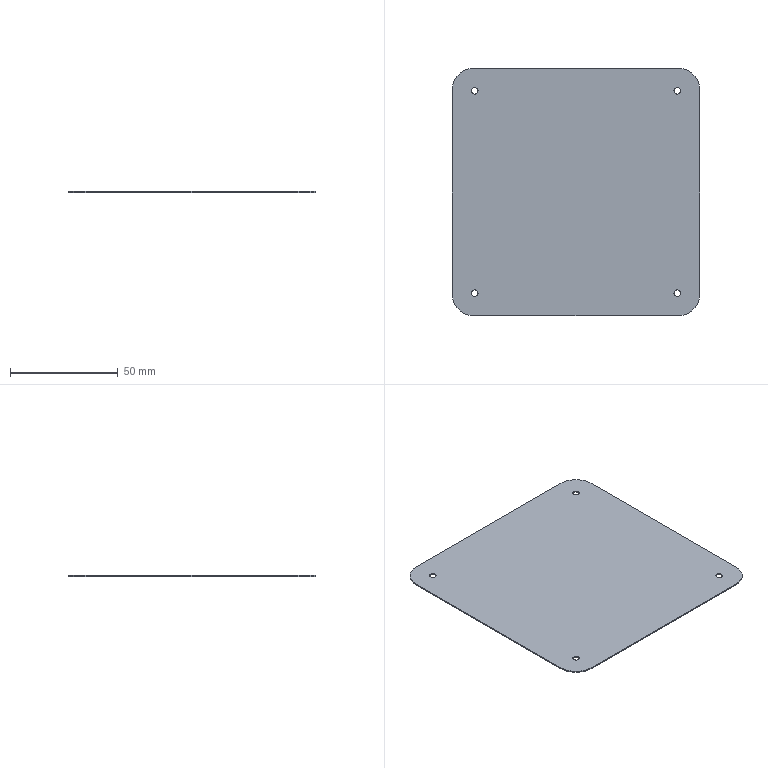Part | SolidWorks | features Extrusion 1 | 1 solid | 18 faces | box 115 x 115 x 0.5 mm | volume 6555 mm3 | cylinder 12 | plane 6 | commonest cylinder face diameters 3 x8 20 x4
STEP:
#1=CARTESIAN_POINT('',(-48.5,-47.,0.5));
#2=VERTEX_POINT('',#1);
#3=CARTESIAN_POINT('',(-45.5,-47.,0.5));
#4=VERTEX_POINT('',#3);
#5=CARTESIAN_POINT('',(-47.,-47.,0.5));
#6=DIRECTION('',(0.,0.,1.));
#7=DIRECTION('',(1.,0.,0.));
#8=AXIS2_PLACEMENT_3D('',#5,#6,#7);
#9=CIRCLE('',#8,1.5);
#10=EDGE_CURVE('',#2,#4,#9,.T.);
#11=ORIENTED_EDGE('',*,*,#10,.T.);
#12=CARTESIAN_POINT('',(-45.5,-47.,0.));
#13=VERTEX_POINT('',#12);
#14=CARTESIAN_POINT('',(-45.5,-47.,0.5));
#15=DIRECTION('',(0.,0.,-1.));
#16=VECTOR('',#15,1000.);
#17=LINE('',#14,#16);
#18=EDGE_CURVE('',#4,#13,#17,.T.);
#19=ORIENTED_EDGE('',*,*,#18,.T.);
#20=CARTESIAN_POINT('',(-48.5,-47.,0.));
#21=VERTEX_POINT('',#20);
#22=CARTESIAN_POINT('',(-47.,-47.,0.));
#23=DIRECTION('',(0.,0.,1.));
#24=DIRECTION('',(1.,0.,0.));
#25=AXIS2_PLACEMENT_3D('',#22,#23,#24);
#26=CIRCLE('',#25,1.5);
#27=EDGE_CURVE('',#21,#13,#26,.T.);
#28=ORIENTED_EDGE('',*,*,#27,.F.);
#29=CARTESIAN_POINT('',(-48.5,-47.,0.5));
#30=DIRECTION('',(0.,0.,-1.));
#31=VECTOR('',#30,1000.);
#32=LINE('',#29,#31);
#33=EDGE_CURVE('',#2,#21,#32,.T.);
#34=ORIENTED_EDGE('',*,*,#33,.F.);
#35=EDGE_LOOP('',(#11,#19,#28,#34));
#36=FACE_OUTER_BOUND('',#35,.T.);
#37=CARTESIAN_POINT('',(-47.,-47.,0.5));
#38=DIRECTION('',(0.,0.,-1.));
#39=DIRECTION('',(-1.,0.,0.));
#40=AXIS2_PLACEMENT_3D('',#37,#38,#39);
#41=CYLINDRICAL_SURFACE('',#40,1.5);
#42=ADVANCED_FACE('',(#36),#41,.F.);
#43=CARTESIAN_POINT('',(45.5,-47.,0.5));
#44=VERTEX_POINT('',#43);
#45=CARTESIAN_POINT('',(48.5,-47.,0.5));
#46=VERTEX_POINT('',#45);
#47=CARTESIAN_POINT('',(47.,-47.,0.5));
#48=DIRECTION('',(0.,0.,1.));
#49=DIRECTION('',(1.,0.,0.));
#50=AXIS2_PLACEMENT_3D('',#47,#48,#49);
#51=CIRCLE('',#50,1.5);
#52=EDGE_CURVE('',#44,#46,#51,.T.);
#53=ORIENTED_EDGE('',*,*,#52,.T.);
#54=CARTESIAN_POINT('',(48.5,-47.,0.));
#55=VERTEX_POINT('',#54);
#56=CARTESIAN_POINT('',(48.5,-47.,0.5));
#57=DIRECTION('',(0.,0.,-1.));
#58=VECTOR('',#57,1000.);
#59=LINE('',#56,#58);
#60=EDGE_CURVE('',#46,#55,#59,.T.);
#61=ORIENTED_EDGE('',*,*,#60,.T.);
#62=CARTESIAN_POINT('',(45.5,-47.,0.));
#63=VERTEX_POINT('',#62);
#64=CARTESIAN_POINT('',(47.,-47.,0.));
#65=DIRECTION('',(0.,0.,1.));
#66=DIRECTION('',(1.,0.,0.));
#67=AXIS2_PLACEMENT_3D('',#64,#65,#66);
#68=CIRCLE('',#67,1.5);
#69=EDGE_CURVE('',#63,#55,#68,.T.);
#70=ORIENTED_EDGE('',*,*,#69,.F.);
#71=CARTESIAN_POINT('',(45.5,-47.,0.5));
#72=DIRECTION('',(0.,0.,-1.));
#73=VECTOR('',#72,1000.);
#74=LINE('',#71,#73);
#75=EDGE_CURVE('',#44,#63,#74,.T.);
#76=ORIENTED_EDGE('',*,*,#75,.F.);
#77=EDGE_LOOP('',(#53,#61,#70,#76));
#78=FACE_OUTER_BOUND('',#77,.T.);
#79=CARTESIAN_POINT('',(47.,-47.,0.5));
#80=DIRECTION('',(0.,0.,-1.));
#81=DIRECTION('',(-1.,0.,0.));
#82=AXIS2_PLACEMENT_3D('',#79,#80,#81);
#83=CYLINDRICAL_SURFACE('',#82,1.5);
#84=ADVANCED_FACE('',(#78),#83,.F.);
#85=CARTESIAN_POINT('',(45.5,47.,0.5));
#86=VERTEX_POINT('',#85);
#87=CARTESIAN_POINT('',(48.5,47.,0.5));
#88=VERTEX_POINT('',#87);
#89=CARTESIAN_POINT('',(47.,47.,0.5));
#90=DIRECTION('',(0.,0.,1.));
#91=DIRECTION('',(1.,0.,0.));
#92=AXIS2_PLACEMENT_3D('',#89,#90,#91);
#93=CIRCLE('',#92,1.5);
#94=EDGE_CURVE('',#86,#88,#93,.T.);
#95=ORIENTED_EDGE('',*,*,#94,.T.);
#96=CARTESIAN_POINT('',(48.5,47.,0.));
#97=VERTEX_POINT('',#96);
#98=CARTESIAN_POINT('',(48.5,47.,0.5));
#99=DIRECTION('',(0.,0.,-1.));
#100=VECTOR('',#99,1000.);
#101=LINE('',#98,#100);
#102=EDGE_CURVE('',#88,#97,#101,.T.);
#103=ORIENTED_EDGE('',*,*,#102,.T.);
#104=CARTESIAN_POINT('',(45.5,47.,0.));
#105=VERTEX_POINT('',#104);
#106=CARTESIAN_POINT('',(47.,47.,0.));
#107=DIRECTION('',(0.,0.,1.));
#108=DIRECTION('',(1.,0.,0.));
#109=AXIS2_PLACEMENT_3D('',#106,#107,#108);
#110=CIRCLE('',#109,1.5);
#111=EDGE_CURVE('',#105,#97,#110,.T.);
#112=ORIENTED_EDGE('',*,*,#111,.F.);
#113=CARTESIAN_POINT('',(45.5,47.,0.5));
#114=DIRECTION('',(0.,0.,-1.));
#115=VECTOR('',#114,1000.);
#116=LINE('',#113,#115);
#117=EDGE_CURVE('',#86,#105,#116,.T.);
#118=ORIENTED_EDGE('',*,*,#117,.F.);
#119=EDGE_LOOP('',(#95,#103,#112,#118));
#120=FACE_OUTER_BOUND('',#119,.T.);
#121=CARTESIAN_POINT('',(47.,47.,0.5));
#122=DIRECTION('',(0.,0.,-1.));
#123=DIRECTION('',(-1.,0.,0.));
#124=AXIS2_PLACEMENT_3D('',#121,#122,#123);
#125=CYLINDRICAL_SURFACE('',#124,1.5);
#126=ADVANCED_FACE('',(#120),#125,.F.);
#127=CARTESIAN_POINT('',(-48.5,47.,0.5));
#128=VERTEX_POINT('',#127);
#129=CARTESIAN_POINT('',(-45.5,47.,0.5));
#130=VERTEX_POINT('',#129);
#131=CARTESIAN_POINT('',(-47.,47.,0.5));
#132=DIRECTION('',(0.,0.,1.));
#133=DIRECTION('',(1.,0.,0.));
#134=AXIS2_PLACEMENT_3D('',#131,#132,#133);
#135=CIRCLE('',#134,1.5);
#136=EDGE_CURVE('',#128,#130,#135,.T.);
#137=ORIENTED_EDGE('',*,*,#136,.T.);
#138=CARTESIAN_POINT('',(-45.5,47.,0.));
#139=VERTEX_POINT('',#138);
#140=CARTESIAN_POINT('',(-45.5,47.,0.5));
#141=DIRECTION('',(0.,0.,-1.));
#142=VECTOR('',#141,1000.);
#143=LINE('',#140,#142);
#144=EDGE_CURVE('',#130,#139,#143,.T.);
#145=ORIENTED_EDGE('',*,*,#144,.T.);
#146=CARTESIAN_POINT('',(-48.5,47.,0.));
#147=VERTEX_POINT('',#146);
#148=CARTESIAN_POINT('',(-47.,47.,0.));
#149=DIRECTION('',(0.,0.,1.));
#150=DIRECTION('',(1.,0.,0.));
#151=AXIS2_PLACEMENT_3D('',#148,#149,#150);
#152=CIRCLE('',#151,1.5);
#153=EDGE_CURVE('',#147,#139,#152,.T.);
#154=ORIENTED_EDGE('',*,*,#153,.F.);
#155=CARTESIAN_POINT('',(-48.5,47.,0.5));
#156=DIRECTION('',(0.,0.,-1.));
#157=VECTOR('',#156,1000.);
#158=LINE('',#155,#157);
#159=EDGE_CURVE('',#128,#147,#158,.T.);
#160=ORIENTED_EDGE('',*,*,#159,.F.);
#161=EDGE_LOOP('',(#137,#145,#154,#160));
#162=FACE_OUTER_BOUND('',#161,.T.);
#163=CARTESIAN_POINT('',(-47.,47.,0.5));
#164=DIRECTION('',(0.,0.,-1.));
#165=DIRECTION('',(-1.,0.,0.));
#166=AXIS2_PLACEMENT_3D('',#163,#164,#165);
#167=CYLINDRICAL_SURFACE('',#166,1.5);
#168=ADVANCED_FACE('',(#162),#167,.F.);
#169=ORIENTED_EDGE('',*,*,#52,.F.);
#170=CARTESIAN_POINT('',(47.,-47.,0.5));
#171=DIRECTION('',(0.,0.,1.));
#172=DIRECTION('',(1.,0.,0.));
#173=AXIS2_PLACEMENT_3D('',#170,#171,#172);
#174=CIRCLE('',#173,1.5);
#175=EDGE_CURVE('',#46,#44,#174,.T.);
#176=ORIENTED_EDGE('',*,*,#175,.F.);
#177=EDGE_LOOP('',(#169,#176));
#178=FACE_BOUND('',#177,.T.);
#179=ORIENTED_EDGE('',*,*,#136,.F.);
#180=CARTESIAN_POINT('',(-47.,47.,0.5));
#181=DIRECTION('',(0.,0.,1.));
#182=DIRECTION('',(1.,0.,0.));
#183=AXIS2_PLACEMENT_3D('',#180,#181,#182);
#184=CIRCLE('',#183,1.5);
#185=EDGE_CURVE('',#130,#128,#184,.T.);
#186=ORIENTED_EDGE('',*,*,#185,.F.);
#187=EDGE_LOOP('',(#179,#186));
#188=FACE_BOUND('',#187,.T.);
#189=CARTESIAN_POINT('',(-47.5,57.5,0.5));
#190=VERTEX_POINT('',#189);
#191=CARTESIAN_POINT('',(-57.5,47.5,0.5));
#192=VERTEX_POINT('',#191);
#193=CARTESIAN_POINT('',(-47.5,47.5,0.5));
#194=DIRECTION('',(0.,0.,1.));
#195=DIRECTION('',(1.,0.,0.));
#196=AXIS2_PLACEMENT_3D('',#193,#194,#195);
#197=CIRCLE('',#196,10.);
#198=EDGE_CURVE('',#190,#192,#197,.T.);
#199=ORIENTED_EDGE('',*,*,#198,.T.);
#200=CARTESIAN_POINT('',(-57.5,-47.5,0.5));
#201=VERTEX_POINT('',#200);
#202=CARTESIAN_POINT('',(-57.5,47.5,0.5));
#203=DIRECTION('',(0.,-1.,0.));
#204=VECTOR('',#203,1000.);
#205=LINE('',#202,#204);
#206=EDGE_CURVE('',#192,#201,#205,.T.);
#207=ORIENTED_EDGE('',*,*,#206,.T.);
#208=CARTESIAN_POINT('',(-47.5,-57.5,0.5));
#209=VERTEX_POINT('',#208);
#210=CARTESIAN_POINT('',(-47.5,-47.5,0.5));
#211=DIRECTION('',(0.,0.,1.));
#212=DIRECTION('',(-1.,0.,0.));
#213=AXIS2_PLACEMENT_3D('',#210,#211,#212);
#214=CIRCLE('',#213,10.);
#215=EDGE_CURVE('',#201,#209,#214,.T.);
#216=ORIENTED_EDGE('',*,*,#215,.T.);
#217=CARTESIAN_POINT('',(47.5,-57.5,0.5));
#218=VERTEX_POINT('',#217);
#219=CARTESIAN_POINT('',(47.5,-57.5,0.5));
#220=DIRECTION('',(1.,0.,0.));
#221=VECTOR('',#220,1000.);
#222=LINE('',#219,#221);
#223=EDGE_CURVE('',#209,#218,#222,.T.);
#224=ORIENTED_EDGE('',*,*,#223,.T.);
#225=CARTESIAN_POINT('',(57.5,-47.5,0.5));
#226=VERTEX_POINT('',#225);
#227=CARTESIAN_POINT('',(47.5,-47.5,0.5));
#228=DIRECTION('',(0.,0.,1.));
#229=DIRECTION('',(-1.,0.,0.));
#230=AXIS2_PLACEMENT_3D('',#227,#228,#229);
#231=CIRCLE('',#230,10.);
#232=EDGE_CURVE('',#218,#226,#231,.T.);
#233=ORIENTED_EDGE('',*,*,#232,.T.);
#234=CARTESIAN_POINT('',(57.5,47.5,0.5));
#235=VERTEX_POINT('',#234);
#236=CARTESIAN_POINT('',(57.5,47.5,0.5));
#237=DIRECTION('',(0.,1.,0.));
#238=VECTOR('',#237,1000.);
#239=LINE('',#236,#238);
#240=EDGE_CURVE('',#226,#235,#239,.T.);
#241=ORIENTED_EDGE('',*,*,#240,.T.);
#242=CARTESIAN_POINT('',(47.5,57.5,0.5));
#243=VERTEX_POINT('',#242);
#244=CARTESIAN_POINT('',(47.5,47.5,0.5));
#245=DIRECTION('',(0.,0.,1.));
#246=DIRECTION('',(-1.,0.,0.));
#247=AXIS2_PLACEMENT_3D('',#244,#245,#246);
#248=CIRCLE('',#247,10.);
#249=EDGE_CURVE('',#235,#243,#248,.T.);
#250=ORIENTED_EDGE('',*,*,#249,.T.);
#251=CARTESIAN_POINT('',(47.5,57.5,0.5));
#252=DIRECTION('',(-1.,0.,0.));
#253=VECTOR('',#252,1000.);
#254=LINE('',#251,#253);
#255=EDGE_CURVE('',#243,#190,#254,.T.);
#256=ORIENTED_EDGE('',*,*,#255,.T.);
#257=EDGE_LOOP('',(#199,#207,#216,#224,#233,#241,#250,#256));
#258=FACE_OUTER_BOUND('',#257,.T.);
#259=ORIENTED_EDGE('',*,*,#94,.F.);
#260=CARTESIAN_POINT('',(47.,47.,0.5));
#261=DIRECTION('',(0.,0.,1.));
#262=DIRECTION('',(1.,0.,0.));
#263=AXIS2_PLACEMENT_3D('',#260,#261,#262);
#264=CIRCLE('',#263,1.5);
#265=EDGE_CURVE('',#88,#86,#264,.T.);
#266=ORIENTED_EDGE('',*,*,#265,.F.);
#267=EDGE_LOOP('',(#259,#266));
#268=FACE_BOUND('',#267,.T.);
#269=ORIENTED_EDGE('',*,*,#10,.F.);
#270=CARTESIAN_POINT('',(-47.,-47.,0.5));
#271=DIRECTION('',(0.,0.,1.));
#272=DIRECTION('',(1.,0.,0.));
#273=AXIS2_PLACEMENT_3D('',#270,#271,#272);
#274=CIRCLE('',#273,1.5);
#275=EDGE_CURVE('',#4,#2,#274,.T.);
#276=ORIENTED_EDGE('',*,*,#275,.F.);
#277=EDGE_LOOP('',(#269,#276));
#278=FACE_BOUND('',#277,.T.);
#279=CARTESIAN_POINT('',(-47.5,47.5,0.5));
#280=DIRECTION('',(0.,0.,1.));
#281=DIRECTION('',(1.,0.,0.));
#282=AXIS2_PLACEMENT_3D('',#279,#280,#281);
#283=PLANE('',#282);
#284=ADVANCED_FACE('',(#178,#188,#258,#268,#278),#283,.T.);
#285=CARTESIAN_POINT('',(-47.5,57.5,0.));
#286=VERTEX_POINT('',#285);
#287=CARTESIAN_POINT('',(-57.5,47.5,0.));
#288=VERTEX_POINT('',#287);
#289=CARTESIAN_POINT('',(-47.5,47.5,0.));
#290=DIRECTION('',(0.,0.,1.));
#291=DIRECTION('',(1.,0.,0.));
#292=AXIS2_PLACEMENT_3D('',#289,#290,#291);
#293=CIRCLE('',#292,10.);
#294=EDGE_CURVE('',#286,#288,#293,.T.);
#295=ORIENTED_EDGE('',*,*,#294,.F.);
#296=CARTESIAN_POINT('',(47.5,57.5,0.));
#297=VERTEX_POINT('',#296);
#298=CARTESIAN_POINT('',(47.5,57.5,0.));
#299=DIRECTION('',(-1.,0.,0.));
#300=VECTOR('',#299,1000.);
#301=LINE('',#298,#300);
#302=EDGE_CURVE('',#297,#286,#301,.T.);
#303=ORIENTED_EDGE('',*,*,#302,.F.);
#304=CARTESIAN_POINT('',(57.5,47.5,0.));
#305=VERTEX_POINT('',#304);
#306=CARTESIAN_POINT('',(47.5,47.5,0.));
#307=DIRECTION('',(0.,0.,1.));
#308=DIRECTION('',(-1.,0.,0.));
#309=AXIS2_PLACEMENT_3D('',#306,#307,#308);
#310=CIRCLE('',#309,10.);
#311=EDGE_CURVE('',#305,#297,#310,.T.);
#312=ORIENTED_EDGE('',*,*,#311,.F.);
#313=CARTESIAN_POINT('',(57.5,-47.5,0.));
#314=VERTEX_POINT('',#313);
#315=CARTESIAN_POINT('',(57.5,47.5,0.));
#316=DIRECTION('',(0.,1.,0.));
#317=VECTOR('',#316,1000.);
#318=LINE('',#315,#317);
#319=EDGE_CURVE('',#314,#305,#318,.T.);
#320=ORIENTED_EDGE('',*,*,#319,.F.);
#321=CARTESIAN_POINT('',(47.5,-57.5,0.));
#322=VERTEX_POINT('',#321);
#323=CARTESIAN_POINT('',(47.5,-47.5,0.));
#324=DIRECTION('',(0.,0.,1.));
#325=DIRECTION('',(-1.,0.,0.));
#326=AXIS2_PLACEMENT_3D('',#323,#324,#325);
#327=CIRCLE('',#326,10.);
#328=EDGE_CURVE('',#322,#314,#327,.T.);
#329=ORIENTED_EDGE('',*,*,#328,.F.);
#330=CARTESIAN_POINT('',(-47.5,-57.5,0.));
#331=VERTEX_POINT('',#330);
#332=CARTESIAN_POINT('',(47.5,-57.5,0.));
#333=DIRECTION('',(1.,0.,0.));
#334=VECTOR('',#333,1000.);
#335=LINE('',#332,#334);
#336=EDGE_CURVE('',#331,#322,#335,.T.);
#337=ORIENTED_EDGE('',*,*,#336,.F.);
#338=CARTESIAN_POINT('',(-57.5,-47.5,0.));
#339=VERTEX_POINT('',#338);
#340=CARTESIAN_POINT('',(-47.5,-47.5,0.));
#341=DIRECTION('',(0.,0.,1.));
#342=DIRECTION('',(-1.,0.,0.));
#343=AXIS2_PLACEMENT_3D('',#340,#341,#342);
#344=CIRCLE('',#343,10.);
#345=EDGE_CURVE('',#339,#331,#344,.T.);
#346=ORIENTED_EDGE('',*,*,#345,.F.);
#347=CARTESIAN_POINT('',(-57.5,47.5,0.));
#348=DIRECTION('',(0.,-1.,0.));
#349=VECTOR('',#348,1000.);
#350=LINE('',#347,#349);
#351=EDGE_CURVE('',#288,#339,#350,.T.);
#352=ORIENTED_EDGE('',*,*,#351,.F.);
#353=EDGE_LOOP('',(#295,#303,#312,#320,#329,#337,#346,#352));
#354=FACE_OUTER_BOUND('',#353,.T.);
#355=ORIENTED_EDGE('',*,*,#153,.T.);
#356=CARTESIAN_POINT('',(-47.,47.,0.));
#357=DIRECTION('',(0.,0.,1.));
#358=DIRECTION('',(1.,0.,0.));
#359=AXIS2_PLACEMENT_3D('',#356,#357,#358);
#360=CIRCLE('',#359,1.5);
#361=EDGE_CURVE('',#139,#147,#360,.T.);
#362=ORIENTED_EDGE('',*,*,#361,.T.);
#363=EDGE_LOOP('',(#355,#362));
#364=FACE_BOUND('',#363,.T.);
#365=ORIENTED_EDGE('',*,*,#111,.T.);
#366=CARTESIAN_POINT('',(47.,47.,0.));
#367=DIRECTION('',(0.,0.,1.));
#368=DIRECTION('',(1.,0.,0.));
#369=AXIS2_PLACEMENT_3D('',#366,#367,#368);
#370=CIRCLE('',#369,1.5);
#371=EDGE_CURVE('',#97,#105,#370,.T.);
#372=ORIENTED_EDGE('',*,*,#371,.T.);
#373=EDGE_LOOP('',(#365,#372));
#374=FACE_BOUND('',#373,.T.);
#375=ORIENTED_EDGE('',*,*,#69,.T.);
#376=CARTESIAN_POINT('',(47.,-47.,0.));
#377=DIRECTION('',(0.,0.,1.));
#378=DIRECTION('',(1.,0.,0.));
#379=AXIS2_PLACEMENT_3D('',#376,#377,#378);
#380=CIRCLE('',#379,1.5);
#381=EDGE_CURVE('',#55,#63,#380,.T.);
#382=ORIENTED_EDGE('',*,*,#381,.T.);
#383=EDGE_LOOP('',(#375,#382));
#384=FACE_BOUND('',#383,.T.);
#385=ORIENTED_EDGE('',*,*,#27,.T.);
#386=CARTESIAN_POINT('',(-47.,-47.,0.));
#387=DIRECTION('',(0.,0.,1.));
#388=DIRECTION('',(1.,0.,0.));
#389=AXIS2_PLACEMENT_3D('',#386,#387,#388);
#390=CIRCLE('',#389,1.5);
#391=EDGE_CURVE('',#13,#21,#390,.T.);
#392=ORIENTED_EDGE('',*,*,#391,.T.);
#393=EDGE_LOOP('',(#385,#392));
#394=FACE_BOUND('',#393,.T.);
#395=CARTESIAN_POINT('',(-47.5,47.5,0.));
#396=DIRECTION('',(0.,0.,1.));
#397=DIRECTION('',(1.,0.,0.));
#398=AXIS2_PLACEMENT_3D('',#395,#396,#397);
#399=PLANE('',#398);
#400=ADVANCED_FACE('',(#354,#364,#374,#384,#394),#399,.F.);
#401=ORIENTED_EDGE('',*,*,#294,.T.);
#402=CARTESIAN_POINT('',(-57.5,47.5,0.5));
#403=DIRECTION('',(0.,0.,-1.));
#404=VECTOR('',#403,1000.);
#405=LINE('',#402,#404);
#406=EDGE_CURVE('',#192,#288,#405,.T.);
#407=ORIENTED_EDGE('',*,*,#406,.F.);
#408=ORIENTED_EDGE('',*,*,#198,.F.);
#409=CARTESIAN_POINT('',(-47.5,57.5,0.5));
#410=DIRECTION('',(0.,0.,-1.));
#411=VECTOR('',#410,1000.);
#412=LINE('',#409,#411);
#413=EDGE_CURVE('',#190,#286,#412,.T.);
#414=ORIENTED_EDGE('',*,*,#413,.T.);
#415=EDGE_LOOP('',(#401,#407,#408,#414));
#416=FACE_OUTER_BOUND('',#415,.T.);
#417=CARTESIAN_POINT('',(-47.5,47.5,0.5));
#418=DIRECTION('',(0.,0.,-1.));
#419=DIRECTION('',(-1.,0.,0.));
#420=AXIS2_PLACEMENT_3D('',#417,#418,#419);
#421=CYLINDRICAL_SURFACE('',#420,10.);
#422=ADVANCED_FACE('',(#416),#421,.T.);
#423=ORIENTED_EDGE('',*,*,#351,.T.);
#424=CARTESIAN_POINT('',(-57.5,-47.5,0.5));
#425=DIRECTION('',(0.,0.,-1.));
#426=VECTOR('',#425,1000.);
#427=LINE('',#424,#426);
#428=EDGE_CURVE('',#201,#339,#427,.T.);
#429=ORIENTED_EDGE('',*,*,#428,.F.);
#430=ORIENTED_EDGE('',*,*,#206,.F.);
#431=ORIENTED_EDGE('',*,*,#406,.T.);
#432=EDGE_LOOP('',(#423,#429,#430,#431));
#433=FACE_OUTER_BOUND('',#432,.T.);
#434=CARTESIAN_POINT('',(-57.5,47.5,0.5));
#435=DIRECTION('',(1.,0.,0.));
#436=DIRECTION('',(0.,1.,0.));
#437=AXIS2_PLACEMENT_3D('',#434,#435,#436);
#438=PLANE('',#437);
#439=ADVANCED_FACE('',(#433),#438,.F.);
#440=ORIENTED_EDGE('',*,*,#345,.T.);
#441=CARTESIAN_POINT('',(-47.5,-57.5,0.5));
#442=DIRECTION('',(0.,0.,-1.));
#443=VECTOR('',#442,1000.);
#444=LINE('',#441,#443);
#445=EDGE_CURVE('',#209,#331,#444,.T.);
#446=ORIENTED_EDGE('',*,*,#445,.F.);
#447=ORIENTED_EDGE('',*,*,#215,.F.);
#448=ORIENTED_EDGE('',*,*,#428,.T.);
#449=EDGE_LOOP('',(#440,#446,#447,#448));
#450=FACE_OUTER_BOUND('',#449,.T.);
#451=CARTESIAN_POINT('',(-47.5,-47.5,0.5));
#452=DIRECTION('',(0.,0.,-1.));
#453=DIRECTION('',(-1.,0.,0.));
#454=AXIS2_PLACEMENT_3D('',#451,#452,#453);
#455=CYLINDRICAL_SURFACE('',#454,10.);
#456=ADVANCED_FACE('',(#450),#455,.T.);
#457=ORIENTED_EDGE('',*,*,#336,.T.);
#458=CARTESIAN_POINT('',(47.5,-57.5,0.5));
#459=DIRECTION('',(0.,0.,-1.));
#460=VECTOR('',#459,1000.);
#461=LINE('',#458,#460);
#462=EDGE_CURVE('',#218,#322,#461,.T.);
#463=ORIENTED_EDGE('',*,*,#462,.F.);
#464=ORIENTED_EDGE('',*,*,#223,.F.);
#465=ORIENTED_EDGE('',*,*,#445,.T.);
#466=EDGE_LOOP('',(#457,#463,#464,#465));
#467=FACE_OUTER_BOUND('',#466,.T.);
#468=CARTESIAN_POINT('',(47.5,-57.5,0.5));
#469=DIRECTION('',(0.,1.,0.));
#470=DIRECTION('',(-1.,0.,0.));
#471=AXIS2_PLACEMENT_3D('',#468,#469,#470);
#472=PLANE('',#471);
#473=ADVANCED_FACE('',(#467),#472,.F.);
#474=ORIENTED_EDGE('',*,*,#328,.T.);
#475=CARTESIAN_POINT('',(57.5,-47.5,0.5));
#476=DIRECTION('',(0.,0.,-1.));
#477=VECTOR('',#476,1000.);
#478=LINE('',#475,#477);
#479=EDGE_CURVE('',#226,#314,#478,.T.);
#480=ORIENTED_EDGE('',*,*,#479,.F.);
#481=ORIENTED_EDGE('',*,*,#232,.F.);
#482=ORIENTED_EDGE('',*,*,#462,.T.);
#483=EDGE_LOOP('',(#474,#480,#481,#482));
#484=FACE_OUTER_BOUND('',#483,.T.);
#485=CARTESIAN_POINT('',(47.5,-47.5,0.5));
#486=DIRECTION('',(0.,0.,-1.));
#487=DIRECTION('',(-1.,0.,0.));
#488=AXIS2_PLACEMENT_3D('',#485,#486,#487);
#489=CYLINDRICAL_SURFACE('',#488,10.);
#490=ADVANCED_FACE('',(#484),#489,.T.);
#491=ORIENTED_EDGE('',*,*,#319,.T.);
#492=CARTESIAN_POINT('',(57.5,47.5,0.5));
#493=DIRECTION('',(0.,0.,-1.));
#494=VECTOR('',#493,1000.);
#495=LINE('',#492,#494);
#496=EDGE_CURVE('',#235,#305,#495,.T.);
#497=ORIENTED_EDGE('',*,*,#496,.F.);
#498=ORIENTED_EDGE('',*,*,#240,.F.);
#499=ORIENTED_EDGE('',*,*,#479,.T.);
#500=EDGE_LOOP('',(#491,#497,#498,#499));
#501=FACE_OUTER_BOUND('',#500,.T.);
#502=CARTESIAN_POINT('',(57.5,47.5,0.5));
#503=DIRECTION('',(-1.,0.,0.));
#504=DIRECTION('',(0.,-1.,0.));
#505=AXIS2_PLACEMENT_3D('',#502,#503,#504);
#506=PLANE('',#505);
#507=ADVANCED_FACE('',(#501),#506,.F.);
#508=ORIENTED_EDGE('',*,*,#311,.T.);
#509=CARTESIAN_POINT('',(47.5,57.5,0.5));
#510=DIRECTION('',(0.,0.,-1.));
#511=VECTOR('',#510,1000.);
#512=LINE('',#509,#511);
#513=EDGE_CURVE('',#243,#297,#512,.T.);
#514=ORIENTED_EDGE('',*,*,#513,.F.);
#515=ORIENTED_EDGE('',*,*,#249,.F.);
#516=ORIENTED_EDGE('',*,*,#496,.T.);
#517=EDGE_LOOP('',(#508,#514,#515,#516));
#518=FACE_OUTER_BOUND('',#517,.T.);
#519=CARTESIAN_POINT('',(47.5,47.5,0.5));
#520=DIRECTION('',(0.,0.,-1.));
#521=DIRECTION('',(-1.,0.,0.));
#522=AXIS2_PLACEMENT_3D('',#519,#520,#521);
#523=CYLINDRICAL_SURFACE('',#522,10.);
#524=ADVANCED_FACE('',(#518),#523,.T.);
#525=ORIENTED_EDGE('',*,*,#302,.T.);
#526=ORIENTED_EDGE('',*,*,#413,.F.);
#527=ORIENTED_EDGE('',*,*,#255,.F.);
#528=ORIENTED_EDGE('',*,*,#513,.T.);
#529=EDGE_LOOP('',(#525,#526,#527,#528));
#530=FACE_OUTER_BOUND('',#529,.T.);
#531=CARTESIAN_POINT('',(47.5,57.5,0.5));
#532=DIRECTION('',(0.,-1.,0.));
#533=DIRECTION('',(1.,0.,0.));
#534=AXIS2_PLACEMENT_3D('',#531,#532,#533);
#535=PLANE('',#534);
#536=ADVANCED_FACE('',(#530),#535,.F.);
#537=ORIENTED_EDGE('',*,*,#144,.F.);
#538=ORIENTED_EDGE('',*,*,#185,.T.);
#539=ORIENTED_EDGE('',*,*,#159,.T.);
#540=ORIENTED_EDGE('',*,*,#361,.F.);
#541=EDGE_LOOP('',(#537,#538,#539,#540));
#542=FACE_OUTER_BOUND('',#541,.T.);
#543=CARTESIAN_POINT('',(-47.,47.,0.5));
#544=DIRECTION('',(0.,0.,-1.));
#545=DIRECTION('',(-1.,0.,0.));
#546=AXIS2_PLACEMENT_3D('',#543,#544,#545);
#547=CYLINDRICAL_SURFACE('',#546,1.5);
#548=ADVANCED_FACE('',(#542),#547,.F.);
#549=ORIENTED_EDGE('',*,*,#102,.F.);
#550=ORIENTED_EDGE('',*,*,#265,.T.);
#551=ORIENTED_EDGE('',*,*,#117,.T.);
#552=ORIENTED_EDGE('',*,*,#371,.F.);
#553=EDGE_LOOP('',(#549,#550,#551,#552));
#554=FACE_OUTER_BOUND('',#553,.T.);
#555=CARTESIAN_POINT('',(47.,47.,0.5));
#556=DIRECTION('',(0.,0.,-1.));
#557=DIRECTION('',(-1.,0.,0.));
#558=AXIS2_PLACEMENT_3D('',#555,#556,#557);
#559=CYLINDRICAL_SURFACE('',#558,1.5);
#560=ADVANCED_FACE('',(#554),#559,.F.);
#561=ORIENTED_EDGE('',*,*,#60,.F.);
#562=ORIENTED_EDGE('',*,*,#175,.T.);
#563=ORIENTED_EDGE('',*,*,#75,.T.);
#564=ORIENTED_EDGE('',*,*,#381,.F.);
#565=EDGE_LOOP('',(#561,#562,#563,#564));
#566=FACE_OUTER_BOUND('',#565,.T.);
#567=CARTESIAN_POINT('',(47.,-47.,0.5));
#568=DIRECTION('',(0.,0.,-1.));
#569=DIRECTION('',(-1.,0.,0.));
#570=AXIS2_PLACEMENT_3D('',#567,#568,#569);
#571=CYLINDRICAL_SURFACE('',#570,1.5);
#572=ADVANCED_FACE('',(#566),#571,.F.);
#573=ORIENTED_EDGE('',*,*,#18,.F.);
#574=ORIENTED_EDGE('',*,*,#275,.T.);
#575=ORIENTED_EDGE('',*,*,#33,.T.);
#576=ORIENTED_EDGE('',*,*,#391,.F.);
#577=EDGE_LOOP('',(#573,#574,#575,#576));
#578=FACE_OUTER_BOUND('',#577,.T.);
#579=CARTESIAN_POINT('',(-47.,-47.,0.5));
#580=DIRECTION('',(0.,0.,-1.));
#581=DIRECTION('',(-1.,0.,0.));
#582=AXIS2_PLACEMENT_3D('',#579,#580,#581);
#583=CYLINDRICAL_SURFACE('',#582,1.5);
#584=ADVANCED_FACE('',(#578),#583,.F.);
#585=CLOSED_SHELL('',(#42,#84,#126,#168,#284,#400,#422,#439,#456,#473,#490,#507,#524,#536,#548,#560,#572,#584));
#586=MANIFOLD_SOLID_BREP('',#585);
#587=CARTESIAN_POINT('',(0.,0.,0.));
#588=DIRECTION('',(0.,0.,1.));
#589=DIRECTION('',(1.,0.,0.));
#590=AXIS2_PLACEMENT_3D('',#587,#588,#589);
#591=(LENGTH_UNIT()NAMED_UNIT(*)SI_UNIT(.MILLI.,.METRE.));
#592=UNCERTAINTY_MEASURE_WITH_UNIT(LENGTH_MEASURE(0.00001),#591,'','');
#593=(NAMED_UNIT(*)PLANE_ANGLE_UNIT()SI_UNIT($,.RADIAN.));
#594=(NAMED_UNIT(*)SI_UNIT($,.STERADIAN.)SOLID_ANGLE_UNIT());
#595=(GEOMETRIC_REPRESENTATION_CONTEXT(3)GLOBAL_UNCERTAINTY_ASSIGNED_CONTEXT((#592))GLOBAL_UNIT_ASSIGNED_CONTEXT((#591,#593,#594))REPRESENTATION_CONTEXT('',''));
#596=ADVANCED_BREP_SHAPE_REPRESENTATION('',(#586,#590),#595);